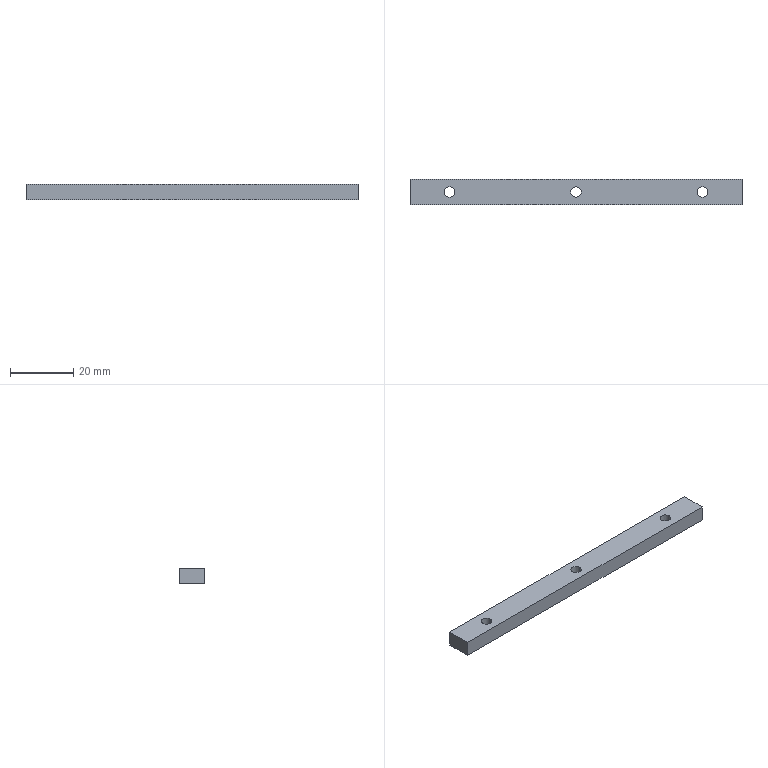Part | SolidWorks | features Extrusion 1, HoleWzd 1 | 1 solid | 12 faces | box 105 x 8 x 5 mm | volume 4072 mm3 | cylinder 6 | plane 6 | commonest cylinder face diameters 3.3 x6
STEP:
#1=CARTESIAN_POINT('',(-41.65,0.,0.));
#2=VERTEX_POINT('',#1);
#3=CARTESIAN_POINT('',(-38.35,0.,0.));
#4=VERTEX_POINT('',#3);
#5=CARTESIAN_POINT('',(-40.,0.,0.));
#6=DIRECTION('',(0.,0.,1.));
#7=DIRECTION('',(1.,0.,0.));
#8=AXIS2_PLACEMENT_3D('',#5,#6,#7);
#9=CIRCLE('',#8,1.65);
#10=EDGE_CURVE('',#2,#4,#9,.T.);
#11=ORIENTED_EDGE('',*,*,#10,.F.);
#12=CARTESIAN_POINT('',(-41.65,0.,5.));
#13=VERTEX_POINT('',#12);
#14=CARTESIAN_POINT('',(-41.65,0.,5.));
#15=DIRECTION('',(0.,0.,1.));
#16=VECTOR('',#15,1000.);
#17=LINE('',#14,#16);
#18=EDGE_CURVE('',#2,#13,#17,.T.);
#19=ORIENTED_EDGE('',*,*,#18,.T.);
#20=CARTESIAN_POINT('',(-38.35,0.,5.));
#21=VERTEX_POINT('',#20);
#22=CARTESIAN_POINT('',(-40.,0.,5.));
#23=DIRECTION('',(0.,0.,1.));
#24=DIRECTION('',(1.,0.,0.));
#25=AXIS2_PLACEMENT_3D('',#22,#23,#24);
#26=CIRCLE('',#25,1.65);
#27=EDGE_CURVE('',#13,#21,#26,.T.);
#28=ORIENTED_EDGE('',*,*,#27,.T.);
#29=CARTESIAN_POINT('',(-38.35,0.,5.));
#30=DIRECTION('',(0.,0.,1.));
#31=VECTOR('',#30,1000.);
#32=LINE('',#29,#31);
#33=EDGE_CURVE('',#4,#21,#32,.T.);
#34=ORIENTED_EDGE('',*,*,#33,.F.);
#35=EDGE_LOOP('',(#11,#19,#28,#34));
#36=FACE_OUTER_BOUND('',#35,.T.);
#37=CARTESIAN_POINT('',(-40.,0.,5.));
#38=DIRECTION('',(0.,0.,1.));
#39=DIRECTION('',(1.,0.,0.));
#40=AXIS2_PLACEMENT_3D('',#37,#38,#39);
#41=CYLINDRICAL_SURFACE('',#40,1.65);
#42=ADVANCED_FACE('',(#36),#41,.F.);
#43=CARTESIAN_POINT('',(-1.65,0.,0.));
#44=VERTEX_POINT('',#43);
#45=CARTESIAN_POINT('',(1.65,0.,0.));
#46=VERTEX_POINT('',#45);
#47=CARTESIAN_POINT('',(0.,0.,0.));
#48=DIRECTION('',(0.,0.,1.));
#49=DIRECTION('',(1.,0.,0.));
#50=AXIS2_PLACEMENT_3D('',#47,#48,#49);
#51=CIRCLE('',#50,1.65);
#52=EDGE_CURVE('',#44,#46,#51,.T.);
#53=ORIENTED_EDGE('',*,*,#52,.F.);
#54=CARTESIAN_POINT('',(-1.65,0.,5.));
#55=VERTEX_POINT('',#54);
#56=CARTESIAN_POINT('',(-1.65,0.,5.));
#57=DIRECTION('',(0.,0.,1.));
#58=VECTOR('',#57,1000.);
#59=LINE('',#56,#58);
#60=EDGE_CURVE('',#44,#55,#59,.T.);
#61=ORIENTED_EDGE('',*,*,#60,.T.);
#62=CARTESIAN_POINT('',(1.65,0.,5.));
#63=VERTEX_POINT('',#62);
#64=CARTESIAN_POINT('',(0.,0.,5.));
#65=DIRECTION('',(0.,0.,1.));
#66=DIRECTION('',(1.,0.,0.));
#67=AXIS2_PLACEMENT_3D('',#64,#65,#66);
#68=CIRCLE('',#67,1.65);
#69=EDGE_CURVE('',#55,#63,#68,.T.);
#70=ORIENTED_EDGE('',*,*,#69,.T.);
#71=CARTESIAN_POINT('',(1.65,0.,5.));
#72=DIRECTION('',(0.,0.,1.));
#73=VECTOR('',#72,1000.);
#74=LINE('',#71,#73);
#75=EDGE_CURVE('',#46,#63,#74,.T.);
#76=ORIENTED_EDGE('',*,*,#75,.F.);
#77=EDGE_LOOP('',(#53,#61,#70,#76));
#78=FACE_OUTER_BOUND('',#77,.T.);
#79=CARTESIAN_POINT('',(0.,0.,5.));
#80=DIRECTION('',(0.,0.,1.));
#81=DIRECTION('',(1.,0.,0.));
#82=AXIS2_PLACEMENT_3D('',#79,#80,#81);
#83=CYLINDRICAL_SURFACE('',#82,1.65);
#84=ADVANCED_FACE('',(#78),#83,.F.);
#85=CARTESIAN_POINT('',(38.35,0.,0.));
#86=VERTEX_POINT('',#85);
#87=CARTESIAN_POINT('',(41.65,0.,0.));
#88=VERTEX_POINT('',#87);
#89=CARTESIAN_POINT('',(40.,0.,0.));
#90=DIRECTION('',(0.,0.,1.));
#91=DIRECTION('',(1.,0.,0.));
#92=AXIS2_PLACEMENT_3D('',#89,#90,#91);
#93=CIRCLE('',#92,1.65);
#94=EDGE_CURVE('',#86,#88,#93,.T.);
#95=ORIENTED_EDGE('',*,*,#94,.F.);
#96=CARTESIAN_POINT('',(38.35,0.,5.));
#97=VERTEX_POINT('',#96);
#98=CARTESIAN_POINT('',(38.35,0.,5.));
#99=DIRECTION('',(0.,0.,1.));
#100=VECTOR('',#99,1000.);
#101=LINE('',#98,#100);
#102=EDGE_CURVE('',#86,#97,#101,.T.);
#103=ORIENTED_EDGE('',*,*,#102,.T.);
#104=CARTESIAN_POINT('',(41.65,0.,5.));
#105=VERTEX_POINT('',#104);
#106=CARTESIAN_POINT('',(40.,0.,5.));
#107=DIRECTION('',(0.,0.,1.));
#108=DIRECTION('',(1.,0.,0.));
#109=AXIS2_PLACEMENT_3D('',#106,#107,#108);
#110=CIRCLE('',#109,1.65);
#111=EDGE_CURVE('',#97,#105,#110,.T.);
#112=ORIENTED_EDGE('',*,*,#111,.T.);
#113=CARTESIAN_POINT('',(41.65,0.,5.));
#114=DIRECTION('',(0.,0.,1.));
#115=VECTOR('',#114,1000.);
#116=LINE('',#113,#115);
#117=EDGE_CURVE('',#88,#105,#116,.T.);
#118=ORIENTED_EDGE('',*,*,#117,.F.);
#119=EDGE_LOOP('',(#95,#103,#112,#118));
#120=FACE_OUTER_BOUND('',#119,.T.);
#121=CARTESIAN_POINT('',(40.,0.,5.));
#122=DIRECTION('',(0.,0.,1.));
#123=DIRECTION('',(1.,0.,0.));
#124=AXIS2_PLACEMENT_3D('',#121,#122,#123);
#125=CYLINDRICAL_SURFACE('',#124,1.65);
#126=ADVANCED_FACE('',(#120),#125,.F.);
#127=CARTESIAN_POINT('',(52.5,-4.,0.));
#128=VERTEX_POINT('',#127);
#129=CARTESIAN_POINT('',(52.5,4.,0.));
#130=VERTEX_POINT('',#129);
#131=CARTESIAN_POINT('',(52.5,4.,0.));
#132=DIRECTION('',(0.,1.,0.));
#133=VECTOR('',#132,1000.);
#134=LINE('',#131,#133);
#135=EDGE_CURVE('',#128,#130,#134,.T.);
#136=ORIENTED_EDGE('',*,*,#135,.T.);
#137=CARTESIAN_POINT('',(52.5,4.,5.));
#138=VERTEX_POINT('',#137);
#139=CARTESIAN_POINT('',(52.5,4.,5.));
#140=DIRECTION('',(0.,0.,-1.));
#141=VECTOR('',#140,1000.);
#142=LINE('',#139,#141);
#143=EDGE_CURVE('',#138,#130,#142,.T.);
#144=ORIENTED_EDGE('',*,*,#143,.F.);
#145=CARTESIAN_POINT('',(52.5,-4.,5.));
#146=VERTEX_POINT('',#145);
#147=CARTESIAN_POINT('',(52.5,4.,5.));
#148=DIRECTION('',(0.,1.,0.));
#149=VECTOR('',#148,1000.);
#150=LINE('',#147,#149);
#151=EDGE_CURVE('',#146,#138,#150,.T.);
#152=ORIENTED_EDGE('',*,*,#151,.F.);
#153=CARTESIAN_POINT('',(52.5,-4.,5.));
#154=DIRECTION('',(0.,0.,-1.));
#155=VECTOR('',#154,1000.);
#156=LINE('',#153,#155);
#157=EDGE_CURVE('',#146,#128,#156,.T.);
#158=ORIENTED_EDGE('',*,*,#157,.T.);
#159=EDGE_LOOP('',(#136,#144,#152,#158));
#160=FACE_OUTER_BOUND('',#159,.T.);
#161=CARTESIAN_POINT('',(52.5,4.,5.));
#162=DIRECTION('',(-1.,0.,0.));
#163=DIRECTION('',(0.,0.,1.));
#164=AXIS2_PLACEMENT_3D('',#161,#162,#163);
#165=PLANE('',#164);
#166=ADVANCED_FACE('',(#160),#165,.F.);
#167=CARTESIAN_POINT('',(-52.5,4.,0.));
#168=VERTEX_POINT('',#167);
#169=CARTESIAN_POINT('',(-52.5,4.,0.));
#170=DIRECTION('',(-1.,0.,0.));
#171=VECTOR('',#170,1000.);
#172=LINE('',#169,#171);
#173=EDGE_CURVE('',#130,#168,#172,.T.);
#174=ORIENTED_EDGE('',*,*,#173,.T.);
#175=CARTESIAN_POINT('',(-52.5,4.,5.));
#176=VERTEX_POINT('',#175);
#177=CARTESIAN_POINT('',(-52.5,4.,5.));
#178=DIRECTION('',(0.,0.,-1.));
#179=VECTOR('',#178,1000.);
#180=LINE('',#177,#179);
#181=EDGE_CURVE('',#176,#168,#180,.T.);
#182=ORIENTED_EDGE('',*,*,#181,.F.);
#183=CARTESIAN_POINT('',(-52.5,4.,5.));
#184=DIRECTION('',(-1.,0.,0.));
#185=VECTOR('',#184,1000.);
#186=LINE('',#183,#185);
#187=EDGE_CURVE('',#138,#176,#186,.T.);
#188=ORIENTED_EDGE('',*,*,#187,.F.);
#189=ORIENTED_EDGE('',*,*,#143,.T.);
#190=EDGE_LOOP('',(#174,#182,#188,#189));
#191=FACE_OUTER_BOUND('',#190,.T.);
#192=CARTESIAN_POINT('',(-52.5,4.,5.));
#193=DIRECTION('',(0.,-1.,0.));
#194=DIRECTION('',(0.,0.,-1.));
#195=AXIS2_PLACEMENT_3D('',#192,#193,#194);
#196=PLANE('',#195);
#197=ADVANCED_FACE('',(#191),#196,.F.);
#198=CARTESIAN_POINT('',(-52.5,-4.,0.));
#199=VERTEX_POINT('',#198);
#200=CARTESIAN_POINT('',(-52.5,4.,0.));
#201=DIRECTION('',(0.,-1.,0.));
#202=VECTOR('',#201,1000.);
#203=LINE('',#200,#202);
#204=EDGE_CURVE('',#168,#199,#203,.T.);
#205=ORIENTED_EDGE('',*,*,#204,.T.);
#206=CARTESIAN_POINT('',(-52.5,-4.,5.));
#207=VERTEX_POINT('',#206);
#208=CARTESIAN_POINT('',(-52.5,-4.,5.));
#209=DIRECTION('',(0.,0.,-1.));
#210=VECTOR('',#209,1000.);
#211=LINE('',#208,#210);
#212=EDGE_CURVE('',#207,#199,#211,.T.);
#213=ORIENTED_EDGE('',*,*,#212,.F.);
#214=CARTESIAN_POINT('',(-52.5,4.,5.));
#215=DIRECTION('',(0.,-1.,0.));
#216=VECTOR('',#215,1000.);
#217=LINE('',#214,#216);
#218=EDGE_CURVE('',#176,#207,#217,.T.);
#219=ORIENTED_EDGE('',*,*,#218,.F.);
#220=ORIENTED_EDGE('',*,*,#181,.T.);
#221=EDGE_LOOP('',(#205,#213,#219,#220));
#222=FACE_OUTER_BOUND('',#221,.T.);
#223=CARTESIAN_POINT('',(-52.5,4.,5.));
#224=DIRECTION('',(1.,0.,0.));
#225=DIRECTION('',(0.,0.,-1.));
#226=AXIS2_PLACEMENT_3D('',#223,#224,#225);
#227=PLANE('',#226);
#228=ADVANCED_FACE('',(#222),#227,.F.);
#229=CARTESIAN_POINT('',(-52.5,-4.,0.));
#230=DIRECTION('',(1.,0.,0.));
#231=VECTOR('',#230,1000.);
#232=LINE('',#229,#231);
#233=EDGE_CURVE('',#199,#128,#232,.T.);
#234=ORIENTED_EDGE('',*,*,#233,.T.);
#235=ORIENTED_EDGE('',*,*,#157,.F.);
#236=CARTESIAN_POINT('',(-52.5,-4.,5.));
#237=DIRECTION('',(1.,0.,0.));
#238=VECTOR('',#237,1000.);
#239=LINE('',#236,#238);
#240=EDGE_CURVE('',#207,#146,#239,.T.);
#241=ORIENTED_EDGE('',*,*,#240,.F.);
#242=ORIENTED_EDGE('',*,*,#212,.T.);
#243=EDGE_LOOP('',(#234,#235,#241,#242));
#244=FACE_OUTER_BOUND('',#243,.T.);
#245=CARTESIAN_POINT('',(-52.5,-4.,5.));
#246=DIRECTION('',(0.,1.,0.));
#247=DIRECTION('',(0.,0.,1.));
#248=AXIS2_PLACEMENT_3D('',#245,#246,#247);
#249=PLANE('',#248);
#250=ADVANCED_FACE('',(#244),#249,.F.);
#251=CARTESIAN_POINT('',(-40.,0.,5.));
#252=DIRECTION('',(0.,0.,1.));
#253=DIRECTION('',(1.,0.,0.));
#254=AXIS2_PLACEMENT_3D('',#251,#252,#253);
#255=CIRCLE('',#254,1.65);
#256=EDGE_CURVE('',#21,#13,#255,.T.);
#257=ORIENTED_EDGE('',*,*,#256,.F.);
#258=ORIENTED_EDGE('',*,*,#27,.F.);
#259=EDGE_LOOP('',(#257,#258));
#260=FACE_BOUND('',#259,.T.);
#261=CARTESIAN_POINT('',(0.,0.,5.));
#262=DIRECTION('',(0.,0.,1.));
#263=DIRECTION('',(1.,0.,0.));
#264=AXIS2_PLACEMENT_3D('',#261,#262,#263);
#265=CIRCLE('',#264,1.65);
#266=EDGE_CURVE('',#63,#55,#265,.T.);
#267=ORIENTED_EDGE('',*,*,#266,.F.);
#268=ORIENTED_EDGE('',*,*,#69,.F.);
#269=EDGE_LOOP('',(#267,#268));
#270=FACE_BOUND('',#269,.T.);
#271=CARTESIAN_POINT('',(40.,0.,5.));
#272=DIRECTION('',(0.,0.,1.));
#273=DIRECTION('',(1.,0.,0.));
#274=AXIS2_PLACEMENT_3D('',#271,#272,#273);
#275=CIRCLE('',#274,1.65);
#276=EDGE_CURVE('',#105,#97,#275,.T.);
#277=ORIENTED_EDGE('',*,*,#276,.F.);
#278=ORIENTED_EDGE('',*,*,#111,.F.);
#279=EDGE_LOOP('',(#277,#278));
#280=FACE_BOUND('',#279,.T.);
#281=ORIENTED_EDGE('',*,*,#151,.T.);
#282=ORIENTED_EDGE('',*,*,#187,.T.);
#283=ORIENTED_EDGE('',*,*,#218,.T.);
#284=ORIENTED_EDGE('',*,*,#240,.T.);
#285=EDGE_LOOP('',(#281,#282,#283,#284));
#286=FACE_OUTER_BOUND('',#285,.T.);
#287=CARTESIAN_POINT('',(0.,0.,5.));
#288=DIRECTION('',(0.,0.,1.));
#289=DIRECTION('',(1.,0.,0.));
#290=AXIS2_PLACEMENT_3D('',#287,#288,#289);
#291=PLANE('',#290);
#292=ADVANCED_FACE('',(#260,#270,#280,#286),#291,.T.);
#293=CARTESIAN_POINT('',(-40.,0.,0.));
#294=DIRECTION('',(0.,0.,1.));
#295=DIRECTION('',(1.,0.,0.));
#296=AXIS2_PLACEMENT_3D('',#293,#294,#295);
#297=CIRCLE('',#296,1.65);
#298=EDGE_CURVE('',#4,#2,#297,.T.);
#299=ORIENTED_EDGE('',*,*,#298,.T.);
#300=ORIENTED_EDGE('',*,*,#10,.T.);
#301=EDGE_LOOP('',(#299,#300));
#302=FACE_BOUND('',#301,.T.);
#303=CARTESIAN_POINT('',(0.,0.,0.));
#304=DIRECTION('',(0.,0.,1.));
#305=DIRECTION('',(1.,0.,0.));
#306=AXIS2_PLACEMENT_3D('',#303,#304,#305);
#307=CIRCLE('',#306,1.65);
#308=EDGE_CURVE('',#46,#44,#307,.T.);
#309=ORIENTED_EDGE('',*,*,#308,.T.);
#310=ORIENTED_EDGE('',*,*,#52,.T.);
#311=EDGE_LOOP('',(#309,#310));
#312=FACE_BOUND('',#311,.T.);
#313=CARTESIAN_POINT('',(40.,0.,0.));
#314=DIRECTION('',(0.,0.,1.));
#315=DIRECTION('',(1.,0.,0.));
#316=AXIS2_PLACEMENT_3D('',#313,#314,#315);
#317=CIRCLE('',#316,1.65);
#318=EDGE_CURVE('',#88,#86,#317,.T.);
#319=ORIENTED_EDGE('',*,*,#318,.T.);
#320=ORIENTED_EDGE('',*,*,#94,.T.);
#321=EDGE_LOOP('',(#319,#320));
#322=FACE_BOUND('',#321,.T.);
#323=ORIENTED_EDGE('',*,*,#135,.F.);
#324=ORIENTED_EDGE('',*,*,#233,.F.);
#325=ORIENTED_EDGE('',*,*,#204,.F.);
#326=ORIENTED_EDGE('',*,*,#173,.F.);
#327=EDGE_LOOP('',(#323,#324,#325,#326));
#328=FACE_OUTER_BOUND('',#327,.T.);
#329=CARTESIAN_POINT('',(0.,0.,0.));
#330=DIRECTION('',(0.,0.,1.));
#331=DIRECTION('',(1.,0.,0.));
#332=AXIS2_PLACEMENT_3D('',#329,#330,#331);
#333=PLANE('',#332);
#334=ADVANCED_FACE('',(#302,#312,#322,#328),#333,.F.);
#335=ORIENTED_EDGE('',*,*,#102,.F.);
#336=ORIENTED_EDGE('',*,*,#318,.F.);
#337=ORIENTED_EDGE('',*,*,#117,.T.);
#338=ORIENTED_EDGE('',*,*,#276,.T.);
#339=EDGE_LOOP('',(#335,#336,#337,#338));
#340=FACE_OUTER_BOUND('',#339,.T.);
#341=CARTESIAN_POINT('',(40.,0.,5.));
#342=DIRECTION('',(0.,0.,1.));
#343=DIRECTION('',(1.,0.,0.));
#344=AXIS2_PLACEMENT_3D('',#341,#342,#343);
#345=CYLINDRICAL_SURFACE('',#344,1.65);
#346=ADVANCED_FACE('',(#340),#345,.F.);
#347=ORIENTED_EDGE('',*,*,#60,.F.);
#348=ORIENTED_EDGE('',*,*,#308,.F.);
#349=ORIENTED_EDGE('',*,*,#75,.T.);
#350=ORIENTED_EDGE('',*,*,#266,.T.);
#351=EDGE_LOOP('',(#347,#348,#349,#350));
#352=FACE_OUTER_BOUND('',#351,.T.);
#353=CARTESIAN_POINT('',(0.,0.,5.));
#354=DIRECTION('',(0.,0.,1.));
#355=DIRECTION('',(1.,0.,0.));
#356=AXIS2_PLACEMENT_3D('',#353,#354,#355);
#357=CYLINDRICAL_SURFACE('',#356,1.65);
#358=ADVANCED_FACE('',(#352),#357,.F.);
#359=ORIENTED_EDGE('',*,*,#18,.F.);
#360=ORIENTED_EDGE('',*,*,#298,.F.);
#361=ORIENTED_EDGE('',*,*,#33,.T.);
#362=ORIENTED_EDGE('',*,*,#256,.T.);
#363=EDGE_LOOP('',(#359,#360,#361,#362));
#364=FACE_OUTER_BOUND('',#363,.T.);
#365=CARTESIAN_POINT('',(-40.,0.,5.));
#366=DIRECTION('',(0.,0.,1.));
#367=DIRECTION('',(1.,0.,0.));
#368=AXIS2_PLACEMENT_3D('',#365,#366,#367);
#369=CYLINDRICAL_SURFACE('',#368,1.65);
#370=ADVANCED_FACE('',(#364),#369,.F.);
#371=CLOSED_SHELL('',(#42,#84,#126,#166,#197,#228,#250,#292,#334,#346,#358,#370));
#372=MANIFOLD_SOLID_BREP('',#371);
#373=CARTESIAN_POINT('',(0.,0.,0.));
#374=DIRECTION('',(0.,0.,1.));
#375=DIRECTION('',(1.,0.,0.));
#376=AXIS2_PLACEMENT_3D('',#373,#374,#375);
#377=(LENGTH_UNIT()NAMED_UNIT(*)SI_UNIT(.MILLI.,.METRE.));
#378=UNCERTAINTY_MEASURE_WITH_UNIT(LENGTH_MEASURE(0.00001),#377,'','');
#379=(NAMED_UNIT(*)PLANE_ANGLE_UNIT()SI_UNIT($,.RADIAN.));
#380=(NAMED_UNIT(*)SI_UNIT($,.STERADIAN.)SOLID_ANGLE_UNIT());
#381=(GEOMETRIC_REPRESENTATION_CONTEXT(3)GLOBAL_UNCERTAINTY_ASSIGNED_CONTEXT((#378))GLOBAL_UNIT_ASSIGNED_CONTEXT((#377,#379,#380))REPRESENTATION_CONTEXT('',''));
#382=ADVANCED_BREP_SHAPE_REPRESENTATION('',(#372,#376),#381);